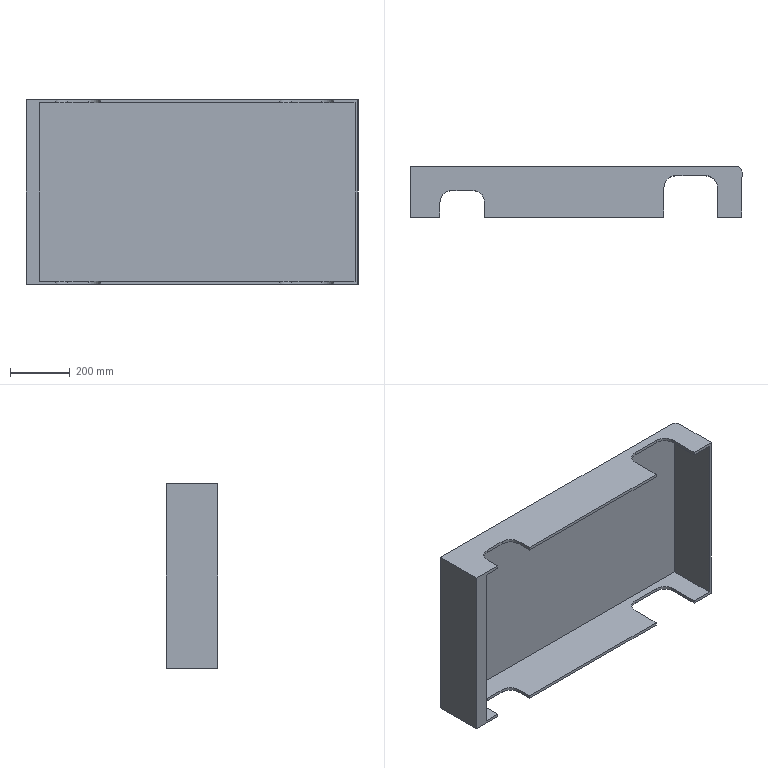Part | SolidWorks | features BaseBody 1 | 1 solid | 35 faces | box 1112 x 170.835 x 618 mm | volume 11764605 mm3 | plane 26 | cylinder 7 | spline 2 | commonest cylinder face diameters 80 x6 40 x1
STEP:
#1=CARTESIAN_POINT('',(484.869,182.944,299.));
#2=VERTEX_POINT('',#1);
#3=CARTESIAN_POINT('',(-571.782,182.944,299.));
#4=VERTEX_POINT('',#3);
#5=CARTESIAN_POINT('',(494.869,182.944,299.));
#6=DIRECTION('',(-1.,0.,0.));
#7=VECTOR('',#6,1000.);
#8=LINE('',#5,#7);
#9=EDGE_CURVE('',#2,#4,#8,.T.);
#10=ORIENTED_EDGE('',*,*,#9,.T.);
#11=CARTESIAN_POINT('',(-571.782,182.944,-299.));
#12=VERTEX_POINT('',#11);
#13=CARTESIAN_POINT('',(-571.782,182.944,-360.));
#14=DIRECTION('',(0.,0.,-1.));
#15=VECTOR('',#14,1000.);
#16=LINE('',#13,#15);
#17=EDGE_CURVE('',#4,#12,#16,.T.);
#18=ORIENTED_EDGE('',*,*,#17,.T.);
#19=CARTESIAN_POINT('',(484.869,182.944,-299.));
#20=VERTEX_POINT('',#19);
#21=CARTESIAN_POINT('',(494.869,182.944,-299.));
#22=DIRECTION('',(-1.,0.,0.));
#23=VECTOR('',#22,1000.);
#24=LINE('',#21,#23);
#25=EDGE_CURVE('',#20,#12,#24,.T.);
#26=ORIENTED_EDGE('',*,*,#25,.F.);
#27=CARTESIAN_POINT('',(484.869,182.944,-360.));
#28=DIRECTION('',(0.,0.,1.));
#29=VECTOR('',#28,1000.);
#30=LINE('',#27,#29);
#31=EDGE_CURVE('',#20,#2,#30,.T.);
#32=ORIENTED_EDGE('',*,*,#31,.T.);
#33=EDGE_LOOP('',(#10,#18,#26,#32));
#34=FACE_OUTER_BOUND('',#33,.T.);
#35=CARTESIAN_POINT('',(494.869,182.944,-360.));
#36=DIRECTION('',(0.,1.,0.));
#37=DIRECTION('',(0.,0.,1.));
#38=AXIS2_PLACEMENT_3D('',#35,#36,#37);
#39=PLANE('',#38);
#40=ADVANCED_FACE('',(#34),#39,.F.);
#41=ORIENTED_EDGE('',*,*,#17,.F.);
#42=CARTESIAN_POINT('',(-571.782,17.142,299.));
#43=VERTEX_POINT('',#42);
#44=CARTESIAN_POINT('',(-571.782,717.138,299.));
#45=DIRECTION('',(0.,-1.,0.));
#46=VECTOR('',#45,1000.);
#47=LINE('',#44,#46);
#48=EDGE_CURVE('',#4,#43,#47,.T.);
#49=ORIENTED_EDGE('',*,*,#48,.T.);
#50=CARTESIAN_POINT('',(-571.782,17.142,-299.));
#51=VERTEX_POINT('',#50);
#52=CARTESIAN_POINT('',(-571.782,17.142,-360.));
#53=DIRECTION('',(0.,0.,1.));
#54=VECTOR('',#53,1000.);
#55=LINE('',#52,#54);
#56=EDGE_CURVE('',#51,#43,#55,.T.);
#57=ORIENTED_EDGE('',*,*,#56,.F.);
#58=CARTESIAN_POINT('',(-571.782,717.138,-299.));
#59=DIRECTION('',(0.,-1.,0.));
#60=VECTOR('',#59,1000.);
#61=LINE('',#58,#60);
#62=EDGE_CURVE('',#12,#51,#61,.T.);
#63=ORIENTED_EDGE('',*,*,#62,.F.);
#64=EDGE_LOOP('',(#41,#49,#57,#63));
#65=FACE_OUTER_BOUND('',#64,.T.);
#66=CARTESIAN_POINT('',(-571.782,717.138,-360.));
#67=DIRECTION('',(-1.,0.,0.));
#68=DIRECTION('',(0.,-1.,0.));
#69=AXIS2_PLACEMENT_3D('',#66,#67,#68);
#70=PLANE('',#69);
#71=ADVANCED_FACE('',(#65),#70,.F.);
#72=CARTESIAN_POINT('',(-616.782,187.944,309.));
#73=VERTEX_POINT('',#72);
#74=CARTESIAN_POINT('',(-616.782,17.108,309.));
#75=VERTEX_POINT('',#74);
#76=CARTESIAN_POINT('',(-616.782,717.138,309.));
#77=DIRECTION('',(0.,-1.,0.));
#78=VECTOR('',#77,1000.);
#79=LINE('',#76,#78);
#80=EDGE_CURVE('',#73,#75,#79,.T.);
#81=ORIENTED_EDGE('',*,*,#80,.F.);
#82=CARTESIAN_POINT('',(-616.782,187.944,-309.));
#83=VERTEX_POINT('',#82);
#84=CARTESIAN_POINT('',(-616.782,187.944,-360.));
#85=DIRECTION('',(0.,0.,-1.));
#86=VECTOR('',#85,1000.);
#87=LINE('',#84,#86);
#88=EDGE_CURVE('',#73,#83,#87,.T.);
#89=ORIENTED_EDGE('',*,*,#88,.T.);
#90=CARTESIAN_POINT('',(-616.782,17.108,-309.));
#91=VERTEX_POINT('',#90);
#92=CARTESIAN_POINT('',(-616.782,717.138,-309.));
#93=DIRECTION('',(0.,-1.,0.));
#94=VECTOR('',#93,1000.);
#95=LINE('',#92,#94);
#96=EDGE_CURVE('',#83,#91,#95,.T.);
#97=ORIENTED_EDGE('',*,*,#96,.T.);
#98=CARTESIAN_POINT('',(-616.782,17.108,-360.));
#99=DIRECTION('',(0.,0.,1.));
#100=VECTOR('',#99,1000.);
#101=LINE('',#98,#100);
#102=EDGE_CURVE('',#91,#75,#101,.T.);
#103=ORIENTED_EDGE('',*,*,#102,.T.);
#104=EDGE_LOOP('',(#81,#89,#97,#103));
#105=FACE_OUTER_BOUND('',#104,.T.);
#106=CARTESIAN_POINT('',(-616.782,717.138,-360.));
#107=DIRECTION('',(-1.,0.,0.));
#108=DIRECTION('',(0.,-1.,0.));
#109=AXIS2_PLACEMENT_3D('',#106,#107,#108);
#110=PLANE('',#109);
#111=ADVANCED_FACE('',(#105),#110,.T.);
#112=CARTESIAN_POINT('',(474.869,187.944,309.));
#113=VERTEX_POINT('',#112);
#114=CARTESIAN_POINT('',(494.869,187.944,309.));
#115=DIRECTION('',(-1.,0.,0.));
#116=VECTOR('',#115,1000.);
#117=LINE('',#114,#116);
#118=EDGE_CURVE('',#113,#73,#117,.T.);
#119=ORIENTED_EDGE('',*,*,#118,.T.);
#120=ORIENTED_EDGE('',*,*,#80,.T.);
#121=CARTESIAN_POINT('',(-516.782,17.183,309.));
#122=VERTEX_POINT('',#121);
#123=CARTESIAN_POINT('',(-576.782,17.138,309.));
#124=DIRECTION('',(1.,0.0007515,0.));
#125=VECTOR('',#124,1000.);
#126=LINE('',#123,#125);
#127=EDGE_CURVE('',#75,#122,#126,.T.);
#128=ORIENTED_EDGE('',*,*,#127,.T.);
#129=CARTESIAN_POINT('',(-516.782,67.138,309.));
#130=VERTEX_POINT('',#129);
#131=CARTESIAN_POINT('',(-516.782,0.,309.));
#132=DIRECTION('',(0.,-1.,0.));
#133=VECTOR('',#132,1000.);
#134=LINE('',#131,#133);
#135=EDGE_CURVE('',#130,#122,#134,.T.);
#136=ORIENTED_EDGE('',*,*,#135,.F.);
#137=CARTESIAN_POINT('',(-476.782,107.138,309.));
#138=VERTEX_POINT('',#137);
#139=CARTESIAN_POINT('',(-476.782,67.138,309.));
#140=DIRECTION('',(0.,0.,1.));
#141=DIRECTION('',(-1.,0.,0.));
#142=AXIS2_PLACEMENT_3D('',#139,#140,#141);
#143=CIRCLE('',#142,40.);
#144=EDGE_CURVE('',#138,#130,#143,.T.);
#145=ORIENTED_EDGE('',*,*,#144,.F.);
#146=CARTESIAN_POINT('',(-406.782,107.138,309.));
#147=VERTEX_POINT('',#146);
#148=CARTESIAN_POINT('',(0.,107.138,309.));
#149=DIRECTION('',(-1.,0.,0.));
#150=VECTOR('',#149,1000.);
#151=LINE('',#148,#150);
#152=EDGE_CURVE('',#147,#138,#151,.T.);
#153=ORIENTED_EDGE('',*,*,#152,.F.);
#154=CARTESIAN_POINT('',(-366.782,67.138,309.));
#155=VERTEX_POINT('',#154);
#156=CARTESIAN_POINT('',(-406.782,67.138,309.));
#157=DIRECTION('',(0.,0.,1.));
#158=DIRECTION('',(-1.,0.,0.));
#159=AXIS2_PLACEMENT_3D('',#156,#157,#158);
#160=CIRCLE('',#159,40.);
#161=EDGE_CURVE('',#155,#147,#160,.T.);
#162=ORIENTED_EDGE('',*,*,#161,.F.);
#163=CARTESIAN_POINT('',(-366.782,17.296,309.));
#164=VERTEX_POINT('',#163);
#165=CARTESIAN_POINT('',(-366.782,0.,309.));
#166=DIRECTION('',(0.,1.,0.));
#167=VECTOR('',#166,1000.);
#168=LINE('',#165,#167);
#169=EDGE_CURVE('',#164,#155,#168,.T.);
#170=ORIENTED_EDGE('',*,*,#169,.F.);
#171=CARTESIAN_POINT('',(233.218,17.747,309.));
#172=VERTEX_POINT('',#171);
#173=CARTESIAN_POINT('',(-576.782,17.138,309.));
#174=DIRECTION('',(1.,0.0007515,0.));
#175=VECTOR('',#174,1000.);
#176=LINE('',#173,#175);
#177=EDGE_CURVE('',#164,#172,#176,.T.);
#178=ORIENTED_EDGE('',*,*,#177,.T.);
#179=CARTESIAN_POINT('',(233.218,117.138,309.));
#180=VERTEX_POINT('',#179);
#181=CARTESIAN_POINT('',(233.218,0.,309.));
#182=DIRECTION('',(0.,-1.,0.));
#183=VECTOR('',#182,1000.);
#184=LINE('',#181,#183);
#185=EDGE_CURVE('',#180,#172,#184,.T.);
#186=ORIENTED_EDGE('',*,*,#185,.F.);
#187=CARTESIAN_POINT('',(273.218,157.138,309.));
#188=VERTEX_POINT('',#187);
#189=CARTESIAN_POINT('',(273.218,117.138,309.));
#190=DIRECTION('',(0.,0.,1.));
#191=DIRECTION('',(-1.,0.,0.));
#192=AXIS2_PLACEMENT_3D('',#189,#190,#191);
#193=CIRCLE('',#192,40.);
#194=EDGE_CURVE('',#188,#180,#193,.T.);
#195=ORIENTED_EDGE('',*,*,#194,.F.);
#196=CARTESIAN_POINT('',(373.218,157.138,309.));
#197=VERTEX_POINT('',#196);
#198=CARTESIAN_POINT('',(0.,157.138,309.));
#199=DIRECTION('',(-1.,0.,0.));
#200=VECTOR('',#199,1000.);
#201=LINE('',#198,#200);
#202=EDGE_CURVE('',#197,#188,#201,.T.);
#203=ORIENTED_EDGE('',*,*,#202,.F.);
#204=CARTESIAN_POINT('',(413.218,117.138,309.));
#205=VERTEX_POINT('',#204);
#206=CARTESIAN_POINT('',(413.218,117.138,309.));
#207=CARTESIAN_POINT('',(413.218,119.8,309.));
#208=CARTESIAN_POINT('',(412.955,122.414,309.));
#209=CARTESIAN_POINT('',(412.185,126.265,309.));
#210=CARTESIAN_POINT('',(411.865,127.537,309.));
#211=CARTESIAN_POINT('',(411.289,129.428,309.));
#212=CARTESIAN_POINT('',(411.08,130.057,309.));
#213=CARTESIAN_POINT('',(410.634,131.297,309.));
#214=CARTESIAN_POINT('',(410.396,131.909,309.));
#215=CARTESIAN_POINT('',(409.139,134.929,309.));
#216=CARTESIAN_POINT('',(407.911,137.217,309.));
#217=CARTESIAN_POINT('',(406.1,139.924,309.));
#218=CARTESIAN_POINT('',(405.724,140.458,309.));
#219=CARTESIAN_POINT('',(404.943,141.51,309.));
#220=CARTESIAN_POINT('',(404.539,142.026,309.));
#221=CARTESIAN_POINT('',(403.297,143.538,309.));
#222=CARTESIAN_POINT('',(402.426,144.498,309.));
#223=CARTESIAN_POINT('',(400.597,146.328,309.));
#224=CARTESIAN_POINT('',(399.639,147.198,309.));
#225=CARTESIAN_POINT('',(397.637,148.846,309.));
#226=CARTESIAN_POINT('',(396.592,149.625,309.));
#227=CARTESIAN_POINT('',(394.41,151.088,309.));
#228=CARTESIAN_POINT('',(393.29,151.762,309.));
#229=CARTESIAN_POINT('',(390.998,152.993,309.));
#230=CARTESIAN_POINT('',(389.824,153.551,309.));
#231=CARTESIAN_POINT('',(387.423,154.554,309.));
#232=CARTESIAN_POINT('',(386.195,154.998,309.));
#233=CARTESIAN_POINT('',(384.311,155.575,309.));
#234=CARTESIAN_POINT('',(383.675,155.753,309.));
#235=CARTESIAN_POINT('',(382.39,156.078,309.));
#236=CARTESIAN_POINT('',(381.744,156.225,309.));
#237=CARTESIAN_POINT('',(378.505,156.875,309.));
#238=CARTESIAN_POINT('',(375.879,157.138,309.));
#239=CARTESIAN_POINT('',(373.218,157.138,309.));
#240=B_SPLINE_CURVE_WITH_KNOTS('',3,(#206,#207,#208,#209,#210,#211,#212,#213,#214,#215,#216,#217,#218,#219,#220,#221,#222,#223,#224,#225,#226,#227,#228,#229,#230,#231,#232,#233,#234,#235,#236,#237,#238,#239),.UNSPECIFIED.,.F.,.F.,(4,2,2,2,2,2,2,2,2,2,2,2,2,2,2,2,4),(0.,0.125,0.1875,0.2187,0.25,0.375,0.4062,0.4375,0.5,0.5625,0.625,0.6875,0.75,0.8125,0.8438,0.875,1.),.UNSPECIFIED.);
#241=EDGE_CURVE('',#205,#197,#240,.T.);
#242=ORIENTED_EDGE('',*,*,#241,.F.);
#243=CARTESIAN_POINT('',(413.218,17.882,309.));
#244=VERTEX_POINT('',#243);
#245=CARTESIAN_POINT('',(413.218,0.,309.));
#246=DIRECTION('',(0.,1.,0.));
#247=VECTOR('',#246,1000.);
#248=LINE('',#245,#247);
#249=EDGE_CURVE('',#244,#205,#248,.T.);
#250=ORIENTED_EDGE('',*,*,#249,.F.);
#251=CARTESIAN_POINT('',(494.869,17.944,309.));
#252=VERTEX_POINT('',#251);
#253=CARTESIAN_POINT('',(-576.782,17.138,309.));
#254=DIRECTION('',(1.,0.0007515,0.));
#255=VECTOR('',#254,1000.);
#256=LINE('',#253,#255);
#257=EDGE_CURVE('',#244,#252,#256,.T.);
#258=ORIENTED_EDGE('',*,*,#257,.T.);
#259=CARTESIAN_POINT('',(494.869,167.944,309.));
#260=VERTEX_POINT('',#259);
#261=CARTESIAN_POINT('',(494.869,17.944,309.));
#262=DIRECTION('',(0.,1.,0.));
#263=VECTOR('',#262,1000.);
#264=LINE('',#261,#263);
#265=EDGE_CURVE('',#252,#260,#264,.T.);
#266=ORIENTED_EDGE('',*,*,#265,.T.);
#267=CARTESIAN_POINT('',(474.869,167.944,309.));
#268=DIRECTION('',(0.,0.,1.));
#269=DIRECTION('',(-1.,0.,0.));
#270=AXIS2_PLACEMENT_3D('',#267,#268,#269);
#271=CIRCLE('',#270,20.);
#272=EDGE_CURVE('',#260,#113,#271,.T.);
#273=ORIENTED_EDGE('',*,*,#272,.T.);
#274=EDGE_LOOP('',(#119,#120,#128,#136,#145,#153,#162,#170,#178,#186,#195,#203,#242,#250,#258,#266,#273));
#275=FACE_OUTER_BOUND('',#274,.T.);
#276=CARTESIAN_POINT('',(0.,0.,309.));
#277=DIRECTION('',(0.,0.,-1.));
#278=DIRECTION('',(-1.,0.,0.));
#279=AXIS2_PLACEMENT_3D('',#276,#277,#278);
#280=PLANE('',#279);
#281=ADVANCED_FACE('',(#275),#280,.F.);
#282=ORIENTED_EDGE('',*,*,#96,.F.);
#283=CARTESIAN_POINT('',(474.869,187.944,-309.));
#284=VERTEX_POINT('',#283);
#285=CARTESIAN_POINT('',(494.869,187.944,-309.));
#286=DIRECTION('',(-1.,0.,0.));
#287=VECTOR('',#286,1000.);
#288=LINE('',#285,#287);
#289=EDGE_CURVE('',#284,#83,#288,.T.);
#290=ORIENTED_EDGE('',*,*,#289,.F.);
#291=CARTESIAN_POINT('',(494.869,167.944,-309.));
#292=VERTEX_POINT('',#291);
#293=CARTESIAN_POINT('',(474.869,167.944,-309.));
#294=DIRECTION('',(0.,0.,-1.));
#295=DIRECTION('',(-1.,0.,0.));
#296=AXIS2_PLACEMENT_3D('',#293,#294,#295);
#297=CIRCLE('',#296,20.);
#298=EDGE_CURVE('',#284,#292,#297,.T.);
#299=ORIENTED_EDGE('',*,*,#298,.T.);
#300=CARTESIAN_POINT('',(494.869,17.944,-309.));
#301=VERTEX_POINT('',#300);
#302=CARTESIAN_POINT('',(494.869,17.944,-309.));
#303=DIRECTION('',(0.,1.,0.));
#304=VECTOR('',#303,1000.);
#305=LINE('',#302,#304);
#306=EDGE_CURVE('',#301,#292,#305,.T.);
#307=ORIENTED_EDGE('',*,*,#306,.F.);
#308=CARTESIAN_POINT('',(413.218,17.882,-309.));
#309=VERTEX_POINT('',#308);
#310=CARTESIAN_POINT('',(-576.782,17.138,-309.));
#311=DIRECTION('',(1.,0.0007515,0.));
#312=VECTOR('',#311,1000.);
#313=LINE('',#310,#312);
#314=EDGE_CURVE('',#309,#301,#313,.T.);
#315=ORIENTED_EDGE('',*,*,#314,.F.);
#316=CARTESIAN_POINT('',(413.218,117.138,-309.));
#317=VERTEX_POINT('',#316);
#318=CARTESIAN_POINT('',(413.218,7.138,-309.));
#319=DIRECTION('',(0.,1.,0.));
#320=VECTOR('',#319,1000.);
#321=LINE('',#318,#320);
#322=EDGE_CURVE('',#309,#317,#321,.T.);
#323=ORIENTED_EDGE('',*,*,#322,.T.);
#324=CARTESIAN_POINT('',(373.218,157.138,-309.));
#325=VERTEX_POINT('',#324);
#326=CARTESIAN_POINT('',(413.218,117.138,-309.));
#327=CARTESIAN_POINT('',(413.218,119.8,-309.));
#328=CARTESIAN_POINT('',(412.955,122.414,-309.));
#329=CARTESIAN_POINT('',(412.185,126.265,-309.));
#330=CARTESIAN_POINT('',(411.865,127.537,-309.));
#331=CARTESIAN_POINT('',(411.289,129.428,-309.));
#332=CARTESIAN_POINT('',(411.08,130.057,-309.));
#333=CARTESIAN_POINT('',(410.634,131.297,-309.));
#334=CARTESIAN_POINT('',(410.396,131.909,-309.));
#335=CARTESIAN_POINT('',(409.139,134.929,-309.));
#336=CARTESIAN_POINT('',(407.911,137.217,-309.));
#337=CARTESIAN_POINT('',(406.1,139.924,-309.));
#338=CARTESIAN_POINT('',(405.724,140.458,-309.));
#339=CARTESIAN_POINT('',(404.943,141.51,-309.));
#340=CARTESIAN_POINT('',(404.539,142.026,-309.));
#341=CARTESIAN_POINT('',(403.297,143.538,-309.));
#342=CARTESIAN_POINT('',(402.426,144.498,-309.));
#343=CARTESIAN_POINT('',(400.597,146.328,-309.));
#344=CARTESIAN_POINT('',(399.639,147.198,-309.));
#345=CARTESIAN_POINT('',(397.637,148.846,-309.));
#346=CARTESIAN_POINT('',(396.592,149.625,-309.));
#347=CARTESIAN_POINT('',(394.41,151.088,-309.));
#348=CARTESIAN_POINT('',(393.29,151.762,-309.));
#349=CARTESIAN_POINT('',(390.998,152.993,-309.));
#350=CARTESIAN_POINT('',(389.824,153.551,-309.));
#351=CARTESIAN_POINT('',(387.423,154.554,-309.));
#352=CARTESIAN_POINT('',(386.195,154.998,-309.));
#353=CARTESIAN_POINT('',(384.311,155.575,-309.));
#354=CARTESIAN_POINT('',(383.675,155.753,-309.));
#355=CARTESIAN_POINT('',(382.39,156.078,-309.));
#356=CARTESIAN_POINT('',(381.744,156.225,-309.));
#357=CARTESIAN_POINT('',(378.505,156.875,-309.));
#358=CARTESIAN_POINT('',(375.879,157.138,-309.));
#359=CARTESIAN_POINT('',(373.218,157.138,-309.));
#360=B_SPLINE_CURVE_WITH_KNOTS('',3,(#326,#327,#328,#329,#330,#331,#332,#333,#334,#335,#336,#337,#338,#339,#340,#341,#342,#343,#344,#345,#346,#347,#348,#349,#350,#351,#352,#353,#354,#355,#356,#357,#358,#359),.UNSPECIFIED.,.F.,.F.,(4,2,2,2,2,2,2,2,2,2,2,2,2,2,2,2,4),(0.,0.125,0.1875,0.2187,0.25,0.375,0.4062,0.4375,0.5,0.5625,0.625,0.6875,0.75,0.8125,0.8438,0.875,1.),.UNSPECIFIED.);
#361=EDGE_CURVE('',#317,#325,#360,.T.);
#362=ORIENTED_EDGE('',*,*,#361,.T.);
#363=CARTESIAN_POINT('',(273.218,157.138,-309.));
#364=VERTEX_POINT('',#363);
#365=CARTESIAN_POINT('',(373.218,157.138,-309.));
#366=DIRECTION('',(-1.,0.,0.));
#367=VECTOR('',#366,1000.);
#368=LINE('',#365,#367);
#369=EDGE_CURVE('',#325,#364,#368,.T.);
#370=ORIENTED_EDGE('',*,*,#369,.T.);
#371=CARTESIAN_POINT('',(233.218,117.138,-309.));
#372=VERTEX_POINT('',#371);
#373=CARTESIAN_POINT('',(273.218,117.138,-309.));
#374=DIRECTION('',(0.,0.,1.));
#375=DIRECTION('',(1.,0.,0.));
#376=AXIS2_PLACEMENT_3D('',#373,#374,#375);
#377=CIRCLE('',#376,40.);
#378=EDGE_CURVE('',#364,#372,#377,.T.);
#379=ORIENTED_EDGE('',*,*,#378,.T.);
#380=CARTESIAN_POINT('',(233.218,17.747,-309.));
#381=VERTEX_POINT('',#380);
#382=CARTESIAN_POINT('',(233.218,17.138,-309.));
#383=DIRECTION('',(0.,-1.,0.));
#384=VECTOR('',#383,1000.);
#385=LINE('',#382,#384);
#386=EDGE_CURVE('',#372,#381,#385,.T.);
#387=ORIENTED_EDGE('',*,*,#386,.T.);
#388=CARTESIAN_POINT('',(-366.782,17.296,-309.));
#389=VERTEX_POINT('',#388);
#390=CARTESIAN_POINT('',(-576.782,17.138,-309.));
#391=DIRECTION('',(1.,0.0007515,0.));
#392=VECTOR('',#391,1000.);
#393=LINE('',#390,#392);
#394=EDGE_CURVE('',#389,#381,#393,.T.);
#395=ORIENTED_EDGE('',*,*,#394,.F.);
#396=CARTESIAN_POINT('',(-366.782,67.138,-309.));
#397=VERTEX_POINT('',#396);
#398=CARTESIAN_POINT('',(-366.782,17.138,-309.));
#399=DIRECTION('',(0.,1.,0.));
#400=VECTOR('',#399,1000.);
#401=LINE('',#398,#400);
#402=EDGE_CURVE('',#389,#397,#401,.T.);
#403=ORIENTED_EDGE('',*,*,#402,.T.);
#404=CARTESIAN_POINT('',(-406.782,107.138,-309.));
#405=VERTEX_POINT('',#404);
#406=CARTESIAN_POINT('',(-406.782,67.138,-309.));
#407=DIRECTION('',(0.,0.,1.));
#408=DIRECTION('',(1.,0.,0.));
#409=AXIS2_PLACEMENT_3D('',#406,#407,#408);
#410=CIRCLE('',#409,40.);
#411=EDGE_CURVE('',#397,#405,#410,.T.);
#412=ORIENTED_EDGE('',*,*,#411,.T.);
#413=CARTESIAN_POINT('',(-476.782,107.138,-309.));
#414=VERTEX_POINT('',#413);
#415=CARTESIAN_POINT('',(-406.782,107.138,-309.));
#416=DIRECTION('',(-1.,0.,0.));
#417=VECTOR('',#416,1000.);
#418=LINE('',#415,#417);
#419=EDGE_CURVE('',#405,#414,#418,.T.);
#420=ORIENTED_EDGE('',*,*,#419,.T.);
#421=CARTESIAN_POINT('',(-516.782,67.138,-309.));
#422=VERTEX_POINT('',#421);
#423=CARTESIAN_POINT('',(-476.782,67.138,-309.));
#424=DIRECTION('',(0.,0.,1.));
#425=DIRECTION('',(1.,0.,0.));
#426=AXIS2_PLACEMENT_3D('',#423,#424,#425);
#427=CIRCLE('',#426,40.);
#428=EDGE_CURVE('',#414,#422,#427,.T.);
#429=ORIENTED_EDGE('',*,*,#428,.T.);
#430=CARTESIAN_POINT('',(-516.782,17.183,-309.));
#431=VERTEX_POINT('',#430);
#432=CARTESIAN_POINT('',(-516.782,17.138,-309.));
#433=DIRECTION('',(0.,-1.,0.));
#434=VECTOR('',#433,1000.);
#435=LINE('',#432,#434);
#436=EDGE_CURVE('',#422,#431,#435,.T.);
#437=ORIENTED_EDGE('',*,*,#436,.T.);
#438=CARTESIAN_POINT('',(-576.782,17.138,-309.));
#439=DIRECTION('',(1.,0.0007515,0.));
#440=VECTOR('',#439,1000.);
#441=LINE('',#438,#440);
#442=EDGE_CURVE('',#91,#431,#441,.T.);
#443=ORIENTED_EDGE('',*,*,#442,.F.);
#444=EDGE_LOOP('',(#282,#290,#299,#307,#315,#323,#362,#370,#379,#387,#395,#403,#412,#420,#429,#437,#443));
#445=FACE_OUTER_BOUND('',#444,.T.);
#446=CARTESIAN_POINT('',(0.,0.,-309.));
#447=DIRECTION('',(0.,0.,-1.));
#448=DIRECTION('',(-1.,0.,0.));
#449=AXIS2_PLACEMENT_3D('',#446,#447,#448);
#450=PLANE('',#449);
#451=ADVANCED_FACE('',(#445),#450,.T.);
#452=ORIENTED_EDGE('',*,*,#25,.T.);
#453=ORIENTED_EDGE('',*,*,#62,.T.);
#454=CARTESIAN_POINT('',(-516.782,17.183,-299.));
#455=VERTEX_POINT('',#454);
#456=CARTESIAN_POINT('',(-576.782,17.138,-299.));
#457=DIRECTION('',(1.,0.0007515,0.));
#458=VECTOR('',#457,1000.);
#459=LINE('',#456,#458);
#460=EDGE_CURVE('',#51,#455,#459,.T.);
#461=ORIENTED_EDGE('',*,*,#460,.T.);
#462=CARTESIAN_POINT('',(-516.782,67.138,-299.));
#463=VERTEX_POINT('',#462);
#464=CARTESIAN_POINT('',(-516.782,0.,-299.));
#465=DIRECTION('',(0.,-1.,0.));
#466=VECTOR('',#465,1000.);
#467=LINE('',#464,#466);
#468=EDGE_CURVE('',#463,#455,#467,.T.);
#469=ORIENTED_EDGE('',*,*,#468,.F.);
#470=CARTESIAN_POINT('',(-476.782,107.138,-299.));
#471=VERTEX_POINT('',#470);
#472=CARTESIAN_POINT('',(-476.782,67.138,-299.));
#473=DIRECTION('',(0.,0.,1.));
#474=DIRECTION('',(-1.,0.,0.));
#475=AXIS2_PLACEMENT_3D('',#472,#473,#474);
#476=CIRCLE('',#475,40.);
#477=EDGE_CURVE('',#471,#463,#476,.T.);
#478=ORIENTED_EDGE('',*,*,#477,.F.);
#479=CARTESIAN_POINT('',(-406.782,107.138,-299.));
#480=VERTEX_POINT('',#479);
#481=CARTESIAN_POINT('',(0.,107.138,-299.));
#482=DIRECTION('',(-1.,0.,0.));
#483=VECTOR('',#482,1000.);
#484=LINE('',#481,#483);
#485=EDGE_CURVE('',#480,#471,#484,.T.);
#486=ORIENTED_EDGE('',*,*,#485,.F.);
#487=CARTESIAN_POINT('',(-366.782,67.138,-299.));
#488=VERTEX_POINT('',#487);
#489=CARTESIAN_POINT('',(-406.782,67.138,-299.));
#490=DIRECTION('',(0.,0.,1.));
#491=DIRECTION('',(-1.,0.,0.));
#492=AXIS2_PLACEMENT_3D('',#489,#490,#491);
#493=CIRCLE('',#492,40.);
#494=EDGE_CURVE('',#488,#480,#493,.T.);
#495=ORIENTED_EDGE('',*,*,#494,.F.);
#496=CARTESIAN_POINT('',(-366.782,17.296,-299.));
#497=VERTEX_POINT('',#496);
#498=CARTESIAN_POINT('',(-366.782,0.,-299.));
#499=DIRECTION('',(0.,1.,0.));
#500=VECTOR('',#499,1000.);
#501=LINE('',#498,#500);
#502=EDGE_CURVE('',#497,#488,#501,.T.);
#503=ORIENTED_EDGE('',*,*,#502,.F.);
#504=CARTESIAN_POINT('',(233.218,17.747,-299.));
#505=VERTEX_POINT('',#504);
#506=CARTESIAN_POINT('',(-576.782,17.138,-299.));
#507=DIRECTION('',(1.,0.0007515,0.));
#508=VECTOR('',#507,1000.);
#509=LINE('',#506,#508);
#510=EDGE_CURVE('',#497,#505,#509,.T.);
#511=ORIENTED_EDGE('',*,*,#510,.T.);
#512=CARTESIAN_POINT('',(233.218,117.138,-299.));
#513=VERTEX_POINT('',#512);
#514=CARTESIAN_POINT('',(233.218,0.,-299.));
#515=DIRECTION('',(0.,-1.,0.));
#516=VECTOR('',#515,1000.);
#517=LINE('',#514,#516);
#518=EDGE_CURVE('',#513,#505,#517,.T.);
#519=ORIENTED_EDGE('',*,*,#518,.F.);
#520=CARTESIAN_POINT('',(273.218,157.138,-299.));
#521=VERTEX_POINT('',#520);
#522=CARTESIAN_POINT('',(273.218,117.138,-299.));
#523=DIRECTION('',(0.,0.,1.));
#524=DIRECTION('',(-1.,0.,0.));
#525=AXIS2_PLACEMENT_3D('',#522,#523,#524);
#526=CIRCLE('',#525,40.);
#527=EDGE_CURVE('',#521,#513,#526,.T.);
#528=ORIENTED_EDGE('',*,*,#527,.F.);
#529=CARTESIAN_POINT('',(373.218,157.138,-299.));
#530=VERTEX_POINT('',#529);
#531=CARTESIAN_POINT('',(0.,157.138,-299.));
#532=DIRECTION('',(-1.,0.,0.));
#533=VECTOR('',#532,1000.);
#534=LINE('',#531,#533);
#535=EDGE_CURVE('',#530,#521,#534,.T.);
#536=ORIENTED_EDGE('',*,*,#535,.F.);
#537=CARTESIAN_POINT('',(413.218,117.138,-299.));
#538=VERTEX_POINT('',#537);
#539=CARTESIAN_POINT('',(413.218,117.138,-299.));
#540=CARTESIAN_POINT('',(413.218,119.761,-299.));
#541=CARTESIAN_POINT('',(412.962,122.351,-299.));
#542=CARTESIAN_POINT('',(412.202,126.191,-299.));
#543=CARTESIAN_POINT('',(411.885,127.463,-299.));
#544=CARTESIAN_POINT('',(411.311,129.358,-299.));
#545=CARTESIAN_POINT('',(411.104,129.985,-299.));
#546=CARTESIAN_POINT('',(410.662,131.222,-299.));
#547=CARTESIAN_POINT('',(410.427,131.832,-299.));
#548=CARTESIAN_POINT('',(409.179,134.848,-299.));
#549=CARTESIAN_POINT('',(407.956,137.14,-299.));
#550=CARTESIAN_POINT('',(406.146,139.857,-299.));
#551=CARTESIAN_POINT('',(405.77,140.393,-299.));
#552=CARTESIAN_POINT('',(404.989,141.45,-299.));
#553=CARTESIAN_POINT('',(404.583,141.971,-299.));
#554=CARTESIAN_POINT('',(403.327,143.505,-299.));
#555=CARTESIAN_POINT('',(402.438,144.486,-299.));
#556=CARTESIAN_POINT('',(399.659,147.267,-299.));
#557=CARTESIAN_POINT('',(397.644,148.922,-299.));
#558=CARTESIAN_POINT('',(394.925,150.742,-299.));
#559=CARTESIAN_POINT('',(394.371,151.094,-299.));
#560=CARTESIAN_POINT('',(393.243,151.771,-299.));
#561=CARTESIAN_POINT('',(392.667,152.098,-299.));
#562=CARTESIAN_POINT('',(390.924,153.03,-299.));
#563=CARTESIAN_POINT('',(389.739,153.59,-299.));
#564=CARTESIAN_POINT('',(386.123,155.089,-299.));
#565=CARTESIAN_POINT('',(383.626,155.85,-299.));
#566=CARTESIAN_POINT('',(380.397,156.494,-299.));
#567=CARTESIAN_POINT('',(379.744,156.608,-299.));
#568=CARTESIAN_POINT('',(378.441,156.802,-299.));
#569=CARTESIAN_POINT('',(376.485,157.043,-299.));
#570=CARTESIAN_POINT('',(374.526,157.138,-299.));
#571=CARTESIAN_POINT('',(373.218,157.138,-299.));
#572=B_SPLINE_CURVE_WITH_KNOTS('',3,(#539,#540,#541,#542,#543,#544,#545,#546,#547,#548,#549,#550,#551,#552,#553,#554,#555,#556,#557,#558,#559,#560,#561,#562,#563,#564,#565,#566,#567,#568,#569,#570,#571),.UNSPECIFIED.,.F.,.F.,(4,2,2,2,2,2,2,2,2,2,2,2,2,2,2,1,4),(0.1304,0.1383,0.1422,0.1442,0.1462,0.154,0.156,0.158,0.1619,0.1698,0.1718,0.1737,0.1777,0.1855,0.1875,0.1895,0.1934),.UNSPECIFIED.);
#573=EDGE_CURVE('',#538,#530,#572,.T.);
#574=ORIENTED_EDGE('',*,*,#573,.F.);
#575=CARTESIAN_POINT('',(413.218,17.882,-299.));
#576=VERTEX_POINT('',#575);
#577=CARTESIAN_POINT('',(413.218,0.,-299.));
#578=DIRECTION('',(0.,1.,0.));
#579=VECTOR('',#578,1000.);
#580=LINE('',#577,#579);
#581=EDGE_CURVE('',#576,#538,#580,.T.);
#582=ORIENTED_EDGE('',*,*,#581,.F.);
#583=CARTESIAN_POINT('',(484.869,17.936,-299.));
#584=VERTEX_POINT('',#583);
#585=CARTESIAN_POINT('',(-576.782,17.138,-299.));
#586=DIRECTION('',(1.,0.0007515,0.));
#587=VECTOR('',#586,1000.);
#588=LINE('',#585,#587);
#589=EDGE_CURVE('',#576,#584,#588,.T.);
#590=ORIENTED_EDGE('',*,*,#589,.T.);
#591=CARTESIAN_POINT('',(484.869,17.944,-299.));
#592=DIRECTION('',(0.,1.,0.));
#593=VECTOR('',#592,1000.);
#594=LINE('',#591,#593);
#595=EDGE_CURVE('',#584,#20,#594,.T.);
#596=ORIENTED_EDGE('',*,*,#595,.T.);
#597=EDGE_LOOP('',(#452,#453,#461,#469,#478,#486,#495,#503,#511,#519,#528,#536,#574,#582,#590,#596));
#598=FACE_OUTER_BOUND('',#597,.T.);
#599=CARTESIAN_POINT('',(0.,0.,-299.));
#600=DIRECTION('',(0.,0.,-1.));
#601=DIRECTION('',(-1.,0.,0.));
#602=AXIS2_PLACEMENT_3D('',#599,#600,#601);
#603=PLANE('',#602);
#604=ADVANCED_FACE('',(#598),#603,.F.);
#605=ORIENTED_EDGE('',*,*,#48,.F.);
#606=ORIENTED_EDGE('',*,*,#9,.F.);
#607=CARTESIAN_POINT('',(484.869,17.936,299.));
#608=VERTEX_POINT('',#607);
#609=CARTESIAN_POINT('',(484.869,17.944,299.));
#610=DIRECTION('',(0.,1.,0.));
#611=VECTOR('',#610,1000.);
#612=LINE('',#609,#611);
#613=EDGE_CURVE('',#608,#2,#612,.T.);
#614=ORIENTED_EDGE('',*,*,#613,.F.);
#615=CARTESIAN_POINT('',(413.218,17.882,299.));
#616=VERTEX_POINT('',#615);
#617=CARTESIAN_POINT('',(-576.782,17.138,299.));
#618=DIRECTION('',(1.,0.0007515,0.));
#619=VECTOR('',#618,1000.);
#620=LINE('',#617,#619);
#621=EDGE_CURVE('',#616,#608,#620,.T.);
#622=ORIENTED_EDGE('',*,*,#621,.F.);
#623=CARTESIAN_POINT('',(413.218,117.138,299.));
#624=VERTEX_POINT('',#623);
#625=CARTESIAN_POINT('',(413.218,0.,299.));
#626=DIRECTION('',(0.,1.,0.));
#627=VECTOR('',#626,1000.);
#628=LINE('',#625,#627);
#629=EDGE_CURVE('',#616,#624,#628,.T.);
#630=ORIENTED_EDGE('',*,*,#629,.T.);
#631=CARTESIAN_POINT('',(373.218,157.138,299.));
#632=VERTEX_POINT('',#631);
#633=CARTESIAN_POINT('',(413.218,117.138,299.));
#634=CARTESIAN_POINT('',(413.218,119.761,299.));
#635=CARTESIAN_POINT('',(412.962,122.351,299.));
#636=CARTESIAN_POINT('',(412.202,126.191,299.));
#637=CARTESIAN_POINT('',(411.885,127.463,299.));
#638=CARTESIAN_POINT('',(411.311,129.358,299.));
#639=CARTESIAN_POINT('',(411.104,129.985,299.));
#640=CARTESIAN_POINT('',(410.662,131.222,299.));
#641=CARTESIAN_POINT('',(410.427,131.832,299.));
#642=CARTESIAN_POINT('',(409.179,134.848,299.));
#643=CARTESIAN_POINT('',(407.956,137.14,299.));
#644=CARTESIAN_POINT('',(406.146,139.857,299.));
#645=CARTESIAN_POINT('',(405.77,140.393,299.));
#646=CARTESIAN_POINT('',(404.989,141.45,299.));
#647=CARTESIAN_POINT('',(404.583,141.971,299.));
#648=CARTESIAN_POINT('',(403.327,143.505,299.));
#649=CARTESIAN_POINT('',(402.438,144.486,299.));
#650=CARTESIAN_POINT('',(399.659,147.267,299.));
#651=CARTESIAN_POINT('',(397.644,148.922,299.));
#652=CARTESIAN_POINT('',(394.925,150.742,299.));
#653=CARTESIAN_POINT('',(394.371,151.094,299.));
#654=CARTESIAN_POINT('',(393.243,151.771,299.));
#655=CARTESIAN_POINT('',(392.667,152.098,299.));
#656=CARTESIAN_POINT('',(390.924,153.03,299.));
#657=CARTESIAN_POINT('',(389.739,153.59,299.));
#658=CARTESIAN_POINT('',(386.123,155.089,299.));
#659=CARTESIAN_POINT('',(383.626,155.85,299.));
#660=CARTESIAN_POINT('',(380.397,156.494,299.));
#661=CARTESIAN_POINT('',(379.744,156.608,299.));
#662=CARTESIAN_POINT('',(378.441,156.802,299.));
#663=CARTESIAN_POINT('',(376.485,157.043,299.));
#664=CARTESIAN_POINT('',(374.526,157.138,299.));
#665=CARTESIAN_POINT('',(373.218,157.138,299.));
#666=B_SPLINE_CURVE_WITH_KNOTS('',3,(#633,#634,#635,#636,#637,#638,#639,#640,#641,#642,#643,#644,#645,#646,#647,#648,#649,#650,#651,#652,#653,#654,#655,#656,#657,#658,#659,#660,#661,#662,#663,#664,#665),.UNSPECIFIED.,.F.,.F.,(4,2,2,2,2,2,2,2,2,2,2,2,2,2,2,1,4),(0.1304,0.1383,0.1422,0.1442,0.1462,0.154,0.156,0.158,0.1619,0.1698,0.1718,0.1737,0.1777,0.1855,0.1875,0.1895,0.1934),.UNSPECIFIED.);
#667=EDGE_CURVE('',#624,#632,#666,.T.);
#668=ORIENTED_EDGE('',*,*,#667,.T.);
#669=CARTESIAN_POINT('',(273.218,157.138,299.));
#670=VERTEX_POINT('',#669);
#671=CARTESIAN_POINT('',(0.,157.138,299.));
#672=DIRECTION('',(-1.,0.,0.));
#673=VECTOR('',#672,1000.);
#674=LINE('',#671,#673);
#675=EDGE_CURVE('',#632,#670,#674,.T.);
#676=ORIENTED_EDGE('',*,*,#675,.T.);
#677=CARTESIAN_POINT('',(233.218,117.138,299.));
#678=VERTEX_POINT('',#677);
#679=CARTESIAN_POINT('',(273.218,117.138,299.));
#680=DIRECTION('',(0.,0.,1.));
#681=DIRECTION('',(-1.,0.,0.));
#682=AXIS2_PLACEMENT_3D('',#679,#680,#681);
#683=CIRCLE('',#682,40.);
#684=EDGE_CURVE('',#670,#678,#683,.T.);
#685=ORIENTED_EDGE('',*,*,#684,.T.);
#686=CARTESIAN_POINT('',(233.218,17.747,299.));
#687=VERTEX_POINT('',#686);
#688=CARTESIAN_POINT('',(233.218,0.,299.));
#689=DIRECTION('',(0.,-1.,0.));
#690=VECTOR('',#689,1000.);
#691=LINE('',#688,#690);
#692=EDGE_CURVE('',#678,#687,#691,.T.);
#693=ORIENTED_EDGE('',*,*,#692,.T.);
#694=CARTESIAN_POINT('',(-366.782,17.296,299.));
#695=VERTEX_POINT('',#694);
#696=CARTESIAN_POINT('',(-576.782,17.138,299.));
#697=DIRECTION('',(1.,0.0007515,0.));
#698=VECTOR('',#697,1000.);
#699=LINE('',#696,#698);
#700=EDGE_CURVE('',#695,#687,#699,.T.);
#701=ORIENTED_EDGE('',*,*,#700,.F.);
#702=CARTESIAN_POINT('',(-366.782,67.138,299.));
#703=VERTEX_POINT('',#702);
#704=CARTESIAN_POINT('',(-366.782,0.,299.));
#705=DIRECTION('',(0.,1.,0.));
#706=VECTOR('',#705,1000.);
#707=LINE('',#704,#706);
#708=EDGE_CURVE('',#695,#703,#707,.T.);
#709=ORIENTED_EDGE('',*,*,#708,.T.);
#710=CARTESIAN_POINT('',(-406.782,107.138,299.));
#711=VERTEX_POINT('',#710);
#712=CARTESIAN_POINT('',(-406.782,67.138,299.));
#713=DIRECTION('',(0.,0.,1.));
#714=DIRECTION('',(-1.,0.,0.));
#715=AXIS2_PLACEMENT_3D('',#712,#713,#714);
#716=CIRCLE('',#715,40.);
#717=EDGE_CURVE('',#703,#711,#716,.T.);
#718=ORIENTED_EDGE('',*,*,#717,.T.);
#719=CARTESIAN_POINT('',(-476.782,107.138,299.));
#720=VERTEX_POINT('',#719);
#721=CARTESIAN_POINT('',(0.,107.138,299.));
#722=DIRECTION('',(-1.,0.,0.));
#723=VECTOR('',#722,1000.);
#724=LINE('',#721,#723);
#725=EDGE_CURVE('',#711,#720,#724,.T.);
#726=ORIENTED_EDGE('',*,*,#725,.T.);
#727=CARTESIAN_POINT('',(-516.782,67.138,299.));
#728=VERTEX_POINT('',#727);
#729=CARTESIAN_POINT('',(-476.782,67.138,299.));
#730=DIRECTION('',(0.,0.,1.));
#731=DIRECTION('',(-1.,0.,0.));
#732=AXIS2_PLACEMENT_3D('',#729,#730,#731);
#733=CIRCLE('',#732,40.);
#734=EDGE_CURVE('',#720,#728,#733,.T.);
#735=ORIENTED_EDGE('',*,*,#734,.T.);
#736=CARTESIAN_POINT('',(-516.782,17.183,299.));
#737=VERTEX_POINT('',#736);
#738=CARTESIAN_POINT('',(-516.782,0.,299.));
#739=DIRECTION('',(0.,-1.,0.));
#740=VECTOR('',#739,1000.);
#741=LINE('',#738,#740);
#742=EDGE_CURVE('',#728,#737,#741,.T.);
#743=ORIENTED_EDGE('',*,*,#742,.T.);
#744=CARTESIAN_POINT('',(-576.782,17.138,299.));
#745=DIRECTION('',(1.,0.0007515,0.));
#746=VECTOR('',#745,1000.);
#747=LINE('',#744,#746);
#748=EDGE_CURVE('',#43,#737,#747,.T.);
#749=ORIENTED_EDGE('',*,*,#748,.F.);
#750=EDGE_LOOP('',(#605,#606,#614,#622,#630,#668,#676,#685,#693,#701,#709,#718,#726,#735,#743,#749));
#751=FACE_OUTER_BOUND('',#750,.T.);
#752=CARTESIAN_POINT('',(0.,0.,299.));
#753=DIRECTION('',(0.,0.,-1.));
#754=DIRECTION('',(-1.,0.,0.));
#755=AXIS2_PLACEMENT_3D('',#752,#753,#754);
#756=PLANE('',#755);
#757=ADVANCED_FACE('',(#751),#756,.T.);
#758=CARTESIAN_POINT('',(-366.782,17.296,-360.));
#759=DIRECTION('',(0.,0.,-1.));
#760=VECTOR('',#759,1000.);
#761=LINE('',#758,#760);
#762=EDGE_CURVE('',#164,#695,#761,.T.);
#763=ORIENTED_EDGE('',*,*,#762,.T.);
#764=ORIENTED_EDGE('',*,*,#700,.T.);
#765=CARTESIAN_POINT('',(233.218,17.747,-360.));
#766=DIRECTION('',(0.,0.,1.));
#767=VECTOR('',#766,1000.);
#768=LINE('',#765,#767);
#769=EDGE_CURVE('',#687,#172,#768,.T.);
#770=ORIENTED_EDGE('',*,*,#769,.T.);
#771=ORIENTED_EDGE('',*,*,#177,.F.);
#772=EDGE_LOOP('',(#763,#764,#770,#771));
#773=FACE_OUTER_BOUND('',#772,.T.);
#774=CARTESIAN_POINT('',(-576.782,17.138,-360.));
#775=DIRECTION('',(0.0007515,-1.,0.));
#776=DIRECTION('',(1.,0.0007515,0.));
#777=AXIS2_PLACEMENT_3D('',#774,#775,#776);
#778=PLANE('',#777);
#779=ADVANCED_FACE('',(#773),#778,.T.);
#780=CARTESIAN_POINT('',(413.218,17.882,-360.));
#781=DIRECTION('',(0.,0.,-1.));
#782=VECTOR('',#781,1000.);
#783=LINE('',#780,#782);
#784=EDGE_CURVE('',#244,#616,#783,.T.);
#785=ORIENTED_EDGE('',*,*,#784,.T.);
#786=ORIENTED_EDGE('',*,*,#621,.T.);
#787=CARTESIAN_POINT('',(484.869,17.936,-360.));
#788=DIRECTION('',(0.,0.,1.));
#789=VECTOR('',#788,1000.);
#790=LINE('',#787,#789);
#791=EDGE_CURVE('',#584,#608,#790,.T.);
#792=ORIENTED_EDGE('',*,*,#791,.F.);
#793=ORIENTED_EDGE('',*,*,#589,.F.);
#794=CARTESIAN_POINT('',(413.218,17.882,-360.));
#795=DIRECTION('',(0.,0.,-1.));
#796=VECTOR('',#795,1000.);
#797=LINE('',#794,#796);
#798=EDGE_CURVE('',#576,#309,#797,.T.);
#799=ORIENTED_EDGE('',*,*,#798,.T.);
#800=ORIENTED_EDGE('',*,*,#314,.T.);
#801=CARTESIAN_POINT('',(494.869,17.944,-360.));
#802=DIRECTION('',(0.,0.,1.));
#803=VECTOR('',#802,1000.);
#804=LINE('',#801,#803);
#805=EDGE_CURVE('',#301,#252,#804,.T.);
#806=ORIENTED_EDGE('',*,*,#805,.T.);
#807=ORIENTED_EDGE('',*,*,#257,.F.);
#808=EDGE_LOOP('',(#785,#786,#792,#793,#799,#800,#806,#807));
#809=FACE_OUTER_BOUND('',#808,.T.);
#810=CARTESIAN_POINT('',(-576.782,17.138,-360.));
#811=DIRECTION('',(0.0007515,-1.,0.));
#812=DIRECTION('',(1.,0.0007515,0.));
#813=AXIS2_PLACEMENT_3D('',#810,#811,#812);
#814=PLANE('',#813);
#815=ADVANCED_FACE('',(#809),#814,.T.);
#816=CARTESIAN_POINT('',(413.218,117.138,2491.));
#817=DIRECTION('',(0.,0.,1.));
#818=VECTOR('',#817,1000.);
#819=LINE('',#816,#818);
#820=EDGE_CURVE('',#317,#538,#819,.T.);
#821=ORIENTED_EDGE('',*,*,#820,.T.);
#822=ORIENTED_EDGE('',*,*,#573,.T.);
#823=CARTESIAN_POINT('',(373.218,157.138,2491.));
#824=DIRECTION('',(0.,0.,1.));
#825=VECTOR('',#824,1000.);
#826=LINE('',#823,#825);
#827=EDGE_CURVE('',#325,#530,#826,.T.);
#828=ORIENTED_EDGE('',*,*,#827,.F.);
#829=ORIENTED_EDGE('',*,*,#361,.F.);
#830=EDGE_LOOP('',(#821,#822,#828,#829));
#831=FACE_OUTER_BOUND('',#830,.T.);
#832=CARTESIAN_POINT('',(413.218,117.138,-299.));
#833=CARTESIAN_POINT('',(413.218,117.138,-309.));
#834=CARTESIAN_POINT('',(413.218,119.8,-299.));
#835=CARTESIAN_POINT('',(413.218,119.8,-309.));
#836=CARTESIAN_POINT('',(412.955,122.414,-299.));
#837=CARTESIAN_POINT('',(412.955,122.414,-309.));
#838=CARTESIAN_POINT('',(412.185,126.265,-299.));
#839=CARTESIAN_POINT('',(412.185,126.265,-309.));
#840=CARTESIAN_POINT('',(411.865,127.537,-299.));
#841=CARTESIAN_POINT('',(411.865,127.537,-309.));
#842=CARTESIAN_POINT('',(411.289,129.428,-299.));
#843=CARTESIAN_POINT('',(411.289,129.428,-309.));
#844=CARTESIAN_POINT('',(411.08,130.057,-299.));
#845=CARTESIAN_POINT('',(411.08,130.057,-309.));
#846=CARTESIAN_POINT('',(410.634,131.297,-299.));
#847=CARTESIAN_POINT('',(410.634,131.297,-309.));
#848=CARTESIAN_POINT('',(410.396,131.909,-299.));
#849=CARTESIAN_POINT('',(410.396,131.909,-309.));
#850=CARTESIAN_POINT('',(409.139,134.929,-299.));
#851=CARTESIAN_POINT('',(409.139,134.929,-309.));
#852=CARTESIAN_POINT('',(407.911,137.217,-299.));
#853=CARTESIAN_POINT('',(407.911,137.217,-309.));
#854=CARTESIAN_POINT('',(406.1,139.924,-299.));
#855=CARTESIAN_POINT('',(406.1,139.924,-309.));
#856=CARTESIAN_POINT('',(405.724,140.458,-299.));
#857=CARTESIAN_POINT('',(405.724,140.458,-309.));
#858=CARTESIAN_POINT('',(404.943,141.51,-299.));
#859=CARTESIAN_POINT('',(404.943,141.51,-309.));
#860=CARTESIAN_POINT('',(404.539,142.026,-299.));
#861=CARTESIAN_POINT('',(404.539,142.026,-309.));
#862=CARTESIAN_POINT('',(403.297,143.538,-299.));
#863=CARTESIAN_POINT('',(403.297,143.538,-309.));
#864=CARTESIAN_POINT('',(402.426,144.498,-299.));
#865=CARTESIAN_POINT('',(402.426,144.498,-309.));
#866=CARTESIAN_POINT('',(400.597,146.328,-299.));
#867=CARTESIAN_POINT('',(400.597,146.328,-309.));
#868=CARTESIAN_POINT('',(399.639,147.198,-299.));
#869=CARTESIAN_POINT('',(399.639,147.198,-309.));
#870=CARTESIAN_POINT('',(397.637,148.846,-299.));
#871=CARTESIAN_POINT('',(397.637,148.846,-309.));
#872=CARTESIAN_POINT('',(396.592,149.625,-299.));
#873=CARTESIAN_POINT('',(396.592,149.625,-309.));
#874=CARTESIAN_POINT('',(394.41,151.088,-299.));
#875=CARTESIAN_POINT('',(394.41,151.088,-309.));
#876=CARTESIAN_POINT('',(393.29,151.762,-299.));
#877=CARTESIAN_POINT('',(393.29,151.762,-309.));
#878=CARTESIAN_POINT('',(390.998,152.993,-299.));
#879=CARTESIAN_POINT('',(390.998,152.993,-309.));
#880=CARTESIAN_POINT('',(389.824,153.551,-299.));
#881=CARTESIAN_POINT('',(389.824,153.551,-309.));
#882=CARTESIAN_POINT('',(387.423,154.554,-299.));
#883=CARTESIAN_POINT('',(387.423,154.554,-309.));
#884=CARTESIAN_POINT('',(386.195,154.998,-299.));
#885=CARTESIAN_POINT('',(386.195,154.998,-309.));
#886=CARTESIAN_POINT('',(384.311,155.575,-299.));
#887=CARTESIAN_POINT('',(384.311,155.575,-309.));
#888=CARTESIAN_POINT('',(383.675,155.753,-299.));
#889=CARTESIAN_POINT('',(383.675,155.753,-309.));
#890=CARTESIAN_POINT('',(382.39,156.078,-299.));
#891=CARTESIAN_POINT('',(382.39,156.078,-309.));
#892=CARTESIAN_POINT('',(381.744,156.225,-299.));
#893=CARTESIAN_POINT('',(381.744,156.225,-309.));
#894=CARTESIAN_POINT('',(378.505,156.875,-299.));
#895=CARTESIAN_POINT('',(378.505,156.875,-309.));
#896=CARTESIAN_POINT('',(375.879,157.138,-299.));
#897=CARTESIAN_POINT('',(375.879,157.138,-309.));
#898=CARTESIAN_POINT('',(373.218,157.138,-299.));
#899=CARTESIAN_POINT('',(373.218,157.138,-309.));
#900=B_SPLINE_SURFACE_WITH_KNOTS('',3,1,((#832,#833),(#834,#835),(#836,#837),(#838,#839),(#840,#841),(#842,#843),(#844,#845),(#846,#847),(#848,#849),(#850,#851),(#852,#853),(#854,#855),(#856,#857),(#858,#859),(#860,#861),(#862,#863),(#864,#865),(#866,#867),(#868,#869),(#870,#871),(#872,#873),(#874,#875),(#876,#877),(#878,#879),(#880,#881),(#882,#883),(#884,#885),(#886,#887),(#888,#889),(#890,#891),(#892,#893),(#894,#895),(#896,#897),(#898,#899)),.UNSPECIFIED.,.F.,.F.,.F.,(4,2,2,2,2,2,2,2,2,2,2,2,2,2,2,2,4),(2,2),(0.,0.125,0.1875,0.2187,0.25,0.375,0.4062,0.4375,0.5,0.5625,0.625,0.6875,0.75,0.8125,0.8438,0.875,1.),(0.,1.),.UNSPECIFIED.);
#901=ADVANCED_FACE('',(#831),#900,.T.);
#902=ORIENTED_EDGE('',*,*,#827,.T.);
#903=ORIENTED_EDGE('',*,*,#535,.T.);
#904=CARTESIAN_POINT('',(273.218,157.138,2491.));
#905=DIRECTION('',(0.,0.,1.));
#906=VECTOR('',#905,1000.);
#907=LINE('',#904,#906);
#908=EDGE_CURVE('',#364,#521,#907,.T.);
#909=ORIENTED_EDGE('',*,*,#908,.F.);
#910=ORIENTED_EDGE('',*,*,#369,.F.);
#911=EDGE_LOOP('',(#902,#903,#909,#910));
#912=FACE_OUTER_BOUND('',#911,.T.);
#913=CARTESIAN_POINT('',(373.218,157.138,2491.));
#914=DIRECTION('',(0.,-1.,0.));
#915=DIRECTION('',(1.,0.,0.));
#916=AXIS2_PLACEMENT_3D('',#913,#914,#915);
#917=PLANE('',#916);
#918=ADVANCED_FACE('',(#912),#917,.T.);
#919=ORIENTED_EDGE('',*,*,#908,.T.);
#920=ORIENTED_EDGE('',*,*,#527,.T.);
#921=CARTESIAN_POINT('',(233.218,117.138,2491.));
#922=DIRECTION('',(0.,0.,1.));
#923=VECTOR('',#922,1000.);
#924=LINE('',#921,#923);
#925=EDGE_CURVE('',#372,#513,#924,.T.);
#926=ORIENTED_EDGE('',*,*,#925,.F.);
#927=ORIENTED_EDGE('',*,*,#378,.F.);
#928=EDGE_LOOP('',(#919,#920,#926,#927));
#929=FACE_OUTER_BOUND('',#928,.T.);
#930=CARTESIAN_POINT('',(273.218,117.138,2491.));
#931=DIRECTION('',(0.,0.,-1.));
#932=DIRECTION('',(-1.,0.,0.));
#933=AXIS2_PLACEMENT_3D('',#930,#931,#932);
#934=CYLINDRICAL_SURFACE('',#933,40.);
#935=ADVANCED_FACE('',(#929),#934,.F.);
#936=ORIENTED_EDGE('',*,*,#798,.F.);
#937=ORIENTED_EDGE('',*,*,#581,.T.);
#938=ORIENTED_EDGE('',*,*,#820,.F.);
#939=ORIENTED_EDGE('',*,*,#322,.F.);
#940=EDGE_LOOP('',(#936,#937,#938,#939));
#941=FACE_OUTER_BOUND('',#940,.T.);
#942=CARTESIAN_POINT('',(413.218,7.138,2491.));
#943=DIRECTION('',(-1.,0.,0.));
#944=DIRECTION('',(0.,0.,1.));
#945=AXIS2_PLACEMENT_3D('',#942,#943,#944);
#946=PLANE('',#945);
#947=ADVANCED_FACE('',(#941),#946,.T.);
#948=ORIENTED_EDGE('',*,*,#925,.T.);
#949=ORIENTED_EDGE('',*,*,#518,.T.);
#950=CARTESIAN_POINT('',(233.218,17.747,-360.));
#951=DIRECTION('',(0.,0.,1.));
#952=VECTOR('',#951,1000.);
#953=LINE('',#950,#952);
#954=EDGE_CURVE('',#381,#505,#953,.T.);
#955=ORIENTED_EDGE('',*,*,#954,.F.);
#956=ORIENTED_EDGE('',*,*,#386,.F.);
#957=EDGE_LOOP('',(#948,#949,#955,#956));
#958=FACE_OUTER_BOUND('',#957,.T.);
#959=CARTESIAN_POINT('',(233.218,17.138,2491.));
#960=DIRECTION('',(1.,0.,0.));
#961=DIRECTION('',(0.,0.,-1.));
#962=AXIS2_PLACEMENT_3D('',#959,#960,#961);
#963=PLANE('',#962);
#964=ADVANCED_FACE('',(#958),#963,.T.);
#965=CARTESIAN_POINT('',(-366.782,67.138,2491.));
#966=DIRECTION('',(0.,0.,1.));
#967=VECTOR('',#966,1000.);
#968=LINE('',#965,#967);
#969=EDGE_CURVE('',#397,#488,#968,.T.);
#970=ORIENTED_EDGE('',*,*,#969,.T.);
#971=ORIENTED_EDGE('',*,*,#494,.T.);
#972=CARTESIAN_POINT('',(-406.782,107.138,2491.));
#973=DIRECTION('',(0.,0.,1.));
#974=VECTOR('',#973,1000.);
#975=LINE('',#972,#974);
#976=EDGE_CURVE('',#405,#480,#975,.T.);
#977=ORIENTED_EDGE('',*,*,#976,.F.);
#978=ORIENTED_EDGE('',*,*,#411,.F.);
#979=EDGE_LOOP('',(#970,#971,#977,#978));
#980=FACE_OUTER_BOUND('',#979,.T.);
#981=CARTESIAN_POINT('',(-406.782,67.138,2491.));
#982=DIRECTION('',(0.,0.,-1.));
#983=DIRECTION('',(-1.,0.,0.));
#984=AXIS2_PLACEMENT_3D('',#981,#982,#983);
#985=CYLINDRICAL_SURFACE('',#984,40.);
#986=ADVANCED_FACE('',(#980),#985,.F.);
#987=ORIENTED_EDGE('',*,*,#976,.T.);
#988=ORIENTED_EDGE('',*,*,#485,.T.);
#989=CARTESIAN_POINT('',(-476.782,107.138,2491.));
#990=DIRECTION('',(0.,0.,1.));
#991=VECTOR('',#990,1000.);
#992=LINE('',#989,#991);
#993=EDGE_CURVE('',#414,#471,#992,.T.);
#994=ORIENTED_EDGE('',*,*,#993,.F.);
#995=ORIENTED_EDGE('',*,*,#419,.F.);
#996=EDGE_LOOP('',(#987,#988,#994,#995));
#997=FACE_OUTER_BOUND('',#996,.T.);
#998=CARTESIAN_POINT('',(-406.782,107.138,2491.));
#999=DIRECTION('',(0.,-1.,0.));
#1000=DIRECTION('',(0.,0.,-1.));
#1001=AXIS2_PLACEMENT_3D('',#998,#999,#1000);
#1002=PLANE('',#1001);
#1003=ADVANCED_FACE('',(#997),#1002,.T.);
#1004=ORIENTED_EDGE('',*,*,#993,.T.);
#1005=ORIENTED_EDGE('',*,*,#477,.T.);
#1006=CARTESIAN_POINT('',(-516.782,67.138,2491.));
#1007=DIRECTION('',(0.,0.,1.));
#1008=VECTOR('',#1007,1000.);
#1009=LINE('',#1006,#1008);
#1010=EDGE_CURVE('',#422,#463,#1009,.T.);
#1011=ORIENTED_EDGE('',*,*,#1010,.F.);
#1012=ORIENTED_EDGE('',*,*,#428,.F.);
#1013=EDGE_LOOP('',(#1004,#1005,#1011,#1012));
#1014=FACE_OUTER_BOUND('',#1013,.T.);
#1015=CARTESIAN_POINT('',(-476.782,67.138,2491.));
#1016=DIRECTION('',(0.,0.,-1.));
#1017=DIRECTION('',(-1.,0.,0.));
#1018=AXIS2_PLACEMENT_3D('',#1015,#1016,#1017);
#1019=CYLINDRICAL_SURFACE('',#1018,40.);
#1020=ADVANCED_FACE('',(#1014),#1019,.F.);
#1021=CARTESIAN_POINT('',(-366.782,17.296,-360.));
#1022=DIRECTION('',(0.,0.,-1.));
#1023=VECTOR('',#1022,1000.);
#1024=LINE('',#1021,#1023);
#1025=EDGE_CURVE('',#497,#389,#1024,.T.);
#1026=ORIENTED_EDGE('',*,*,#1025,.F.);
#1027=ORIENTED_EDGE('',*,*,#502,.T.);
#1028=ORIENTED_EDGE('',*,*,#969,.F.);
#1029=ORIENTED_EDGE('',*,*,#402,.F.);
#1030=EDGE_LOOP('',(#1026,#1027,#1028,#1029));
#1031=FACE_OUTER_BOUND('',#1030,.T.);
#1032=CARTESIAN_POINT('',(-366.782,17.138,2491.));
#1033=DIRECTION('',(-1.,0.,0.));
#1034=DIRECTION('',(0.,0.,1.));
#1035=AXIS2_PLACEMENT_3D('',#1032,#1033,#1034);
#1036=PLANE('',#1035);
#1037=ADVANCED_FACE('',(#1031),#1036,.T.);
#1038=ORIENTED_EDGE('',*,*,#1010,.T.);
#1039=ORIENTED_EDGE('',*,*,#468,.T.);
#1040=CARTESIAN_POINT('',(-516.782,17.183,-360.));
#1041=DIRECTION('',(0.,0.,1.));
#1042=VECTOR('',#1041,1000.);
#1043=LINE('',#1040,#1042);
#1044=EDGE_CURVE('',#431,#455,#1043,.T.);
#1045=ORIENTED_EDGE('',*,*,#1044,.F.);
#1046=ORIENTED_EDGE('',*,*,#436,.F.);
#1047=EDGE_LOOP('',(#1038,#1039,#1045,#1046));
#1048=FACE_OUTER_BOUND('',#1047,.T.);
#1049=CARTESIAN_POINT('',(-516.782,17.138,2491.));
#1050=DIRECTION('',(1.,0.,0.));
#1051=DIRECTION('',(0.,0.,-1.));
#1052=AXIS2_PLACEMENT_3D('',#1049,#1050,#1051);
#1053=PLANE('',#1052);
#1054=ADVANCED_FACE('',(#1048),#1053,.T.);
#1055=ORIENTED_EDGE('',*,*,#510,.F.);
#1056=ORIENTED_EDGE('',*,*,#1025,.T.);
#1057=ORIENTED_EDGE('',*,*,#394,.T.);
#1058=ORIENTED_EDGE('',*,*,#954,.T.);
#1059=EDGE_LOOP('',(#1055,#1056,#1057,#1058));
#1060=FACE_OUTER_BOUND('',#1059,.T.);
#1061=CARTESIAN_POINT('',(-576.782,17.138,-360.));
#1062=DIRECTION('',(0.0007515,-1.,0.));
#1063=DIRECTION('',(1.,0.0007515,0.));
#1064=AXIS2_PLACEMENT_3D('',#1061,#1062,#1063);
#1065=PLANE('',#1064);
#1066=ADVANCED_FACE('',(#1060),#1065,.T.);
#1067=ORIENTED_EDGE('',*,*,#460,.F.);
#1068=ORIENTED_EDGE('',*,*,#56,.T.);
#1069=ORIENTED_EDGE('',*,*,#748,.T.);
#1070=CARTESIAN_POINT('',(-516.782,17.183,-360.));
#1071=DIRECTION('',(0.,0.,1.));
#1072=VECTOR('',#1071,1000.);
#1073=LINE('',#1070,#1072);
#1074=EDGE_CURVE('',#737,#122,#1073,.T.);
#1075=ORIENTED_EDGE('',*,*,#1074,.T.);
#1076=ORIENTED_EDGE('',*,*,#127,.F.);
#1077=ORIENTED_EDGE('',*,*,#102,.F.);
#1078=ORIENTED_EDGE('',*,*,#442,.T.);
#1079=ORIENTED_EDGE('',*,*,#1044,.T.);
#1080=EDGE_LOOP('',(#1067,#1068,#1069,#1075,#1076,#1077,#1078,#1079));
#1081=FACE_OUTER_BOUND('',#1080,.T.);
#1082=CARTESIAN_POINT('',(-576.782,17.138,-360.));
#1083=DIRECTION('',(0.0007515,-1.,0.));
#1084=DIRECTION('',(1.,0.0007515,0.));
#1085=AXIS2_PLACEMENT_3D('',#1082,#1083,#1084);
#1086=PLANE('',#1085);
#1087=ADVANCED_FACE('',(#1081),#1086,.T.);
#1088=ORIENTED_EDGE('',*,*,#306,.T.);
#1089=CARTESIAN_POINT('',(494.869,167.944,-360.));
#1090=DIRECTION('',(0.,0.,1.));
#1091=VECTOR('',#1090,1000.);
#1092=LINE('',#1089,#1091);
#1093=EDGE_CURVE('',#292,#260,#1092,.T.);
#1094=ORIENTED_EDGE('',*,*,#1093,.T.);
#1095=ORIENTED_EDGE('',*,*,#265,.F.);
#1096=ORIENTED_EDGE('',*,*,#805,.F.);
#1097=EDGE_LOOP('',(#1088,#1094,#1095,#1096));
#1098=FACE_OUTER_BOUND('',#1097,.T.);
#1099=CARTESIAN_POINT('',(494.869,17.944,-360.));
#1100=DIRECTION('',(1.,0.,0.));
#1101=DIRECTION('',(0.,1.,0.));
#1102=AXIS2_PLACEMENT_3D('',#1099,#1100,#1101);
#1103=PLANE('',#1102);
#1104=ADVANCED_FACE('',(#1098),#1103,.T.);
#1105=ORIENTED_EDGE('',*,*,#88,.F.);
#1106=ORIENTED_EDGE('',*,*,#118,.F.);
#1107=CARTESIAN_POINT('',(474.869,187.944,-360.));
#1108=DIRECTION('',(0.,0.,-1.));
#1109=VECTOR('',#1108,1000.);
#1110=LINE('',#1107,#1109);
#1111=EDGE_CURVE('',#113,#284,#1110,.T.);
#1112=ORIENTED_EDGE('',*,*,#1111,.T.);
#1113=ORIENTED_EDGE('',*,*,#289,.T.);
#1114=EDGE_LOOP('',(#1105,#1106,#1112,#1113));
#1115=FACE_OUTER_BOUND('',#1114,.T.);
#1116=CARTESIAN_POINT('',(494.869,187.944,-360.));
#1117=DIRECTION('',(0.,1.,0.));
#1118=DIRECTION('',(0.,0.,1.));
#1119=AXIS2_PLACEMENT_3D('',#1116,#1117,#1118);
#1120=PLANE('',#1119);
#1121=ADVANCED_FACE('',(#1115),#1120,.T.);
#1122=ORIENTED_EDGE('',*,*,#667,.F.);
#1123=CARTESIAN_POINT('',(413.218,117.138,2491.));
#1124=DIRECTION('',(0.,0.,1.));
#1125=VECTOR('',#1124,1000.);
#1126=LINE('',#1123,#1125);
#1127=EDGE_CURVE('',#624,#205,#1126,.T.);
#1128=ORIENTED_EDGE('',*,*,#1127,.T.);
#1129=ORIENTED_EDGE('',*,*,#241,.T.);
#1130=CARTESIAN_POINT('',(373.218,157.138,2491.));
#1131=DIRECTION('',(0.,0.,1.));
#1132=VECTOR('',#1131,1000.);
#1133=LINE('',#1130,#1132);
#1134=EDGE_CURVE('',#632,#197,#1133,.T.);
#1135=ORIENTED_EDGE('',*,*,#1134,.F.);
#1136=EDGE_LOOP('',(#1122,#1128,#1129,#1135));
#1137=FACE_OUTER_BOUND('',#1136,.T.);
#1138=CARTESIAN_POINT('',(413.218,117.138,309.));
#1139=CARTESIAN_POINT('',(413.218,117.138,299.));
#1140=CARTESIAN_POINT('',(413.218,119.8,309.));
#1141=CARTESIAN_POINT('',(413.218,119.8,299.));
#1142=CARTESIAN_POINT('',(412.955,122.414,309.));
#1143=CARTESIAN_POINT('',(412.955,122.414,299.));
#1144=CARTESIAN_POINT('',(412.185,126.265,309.));
#1145=CARTESIAN_POINT('',(412.185,126.265,299.));
#1146=CARTESIAN_POINT('',(411.865,127.537,309.));
#1147=CARTESIAN_POINT('',(411.865,127.537,299.));
#1148=CARTESIAN_POINT('',(411.289,129.428,309.));
#1149=CARTESIAN_POINT('',(411.289,129.428,299.));
#1150=CARTESIAN_POINT('',(411.08,130.057,309.));
#1151=CARTESIAN_POINT('',(411.08,130.057,299.));
#1152=CARTESIAN_POINT('',(410.634,131.297,309.));
#1153=CARTESIAN_POINT('',(410.634,131.297,299.));
#1154=CARTESIAN_POINT('',(410.396,131.909,309.));
#1155=CARTESIAN_POINT('',(410.396,131.909,299.));
#1156=CARTESIAN_POINT('',(409.139,134.929,309.));
#1157=CARTESIAN_POINT('',(409.139,134.929,299.));
#1158=CARTESIAN_POINT('',(407.911,137.217,309.));
#1159=CARTESIAN_POINT('',(407.911,137.217,299.));
#1160=CARTESIAN_POINT('',(406.1,139.924,309.));
#1161=CARTESIAN_POINT('',(406.1,139.924,299.));
#1162=CARTESIAN_POINT('',(405.724,140.458,309.));
#1163=CARTESIAN_POINT('',(405.724,140.458,299.));
#1164=CARTESIAN_POINT('',(404.943,141.51,309.));
#1165=CARTESIAN_POINT('',(404.943,141.51,299.));
#1166=CARTESIAN_POINT('',(404.539,142.026,309.));
#1167=CARTESIAN_POINT('',(404.539,142.026,299.));
#1168=CARTESIAN_POINT('',(403.297,143.538,309.));
#1169=CARTESIAN_POINT('',(403.297,143.538,299.));
#1170=CARTESIAN_POINT('',(402.426,144.498,309.));
#1171=CARTESIAN_POINT('',(402.426,144.498,299.));
#1172=CARTESIAN_POINT('',(400.597,146.328,309.));
#1173=CARTESIAN_POINT('',(400.597,146.328,299.));
#1174=CARTESIAN_POINT('',(399.639,147.198,309.));
#1175=CARTESIAN_POINT('',(399.639,147.198,299.));
#1176=CARTESIAN_POINT('',(397.637,148.846,309.));
#1177=CARTESIAN_POINT('',(397.637,148.846,299.));
#1178=CARTESIAN_POINT('',(396.592,149.625,309.));
#1179=CARTESIAN_POINT('',(396.592,149.625,299.));
#1180=CARTESIAN_POINT('',(394.41,151.088,309.));
#1181=CARTESIAN_POINT('',(394.41,151.088,299.));
#1182=CARTESIAN_POINT('',(393.29,151.762,309.));
#1183=CARTESIAN_POINT('',(393.29,151.762,299.));
#1184=CARTESIAN_POINT('',(390.998,152.993,309.));
#1185=CARTESIAN_POINT('',(390.998,152.993,299.));
#1186=CARTESIAN_POINT('',(389.824,153.551,309.));
#1187=CARTESIAN_POINT('',(389.824,153.551,299.));
#1188=CARTESIAN_POINT('',(387.423,154.554,309.));
#1189=CARTESIAN_POINT('',(387.423,154.554,299.));
#1190=CARTESIAN_POINT('',(386.195,154.998,309.));
#1191=CARTESIAN_POINT('',(386.195,154.998,299.));
#1192=CARTESIAN_POINT('',(384.311,155.575,309.));
#1193=CARTESIAN_POINT('',(384.311,155.575,299.));
#1194=CARTESIAN_POINT('',(383.675,155.753,309.));
#1195=CARTESIAN_POINT('',(383.675,155.753,299.));
#1196=CARTESIAN_POINT('',(382.39,156.078,309.));
#1197=CARTESIAN_POINT('',(382.39,156.078,299.));
#1198=CARTESIAN_POINT('',(381.744,156.225,309.));
#1199=CARTESIAN_POINT('',(381.744,156.225,299.));
#1200=CARTESIAN_POINT('',(378.505,156.875,309.));
#1201=CARTESIAN_POINT('',(378.505,156.875,299.));
#1202=CARTESIAN_POINT('',(375.879,157.138,309.));
#1203=CARTESIAN_POINT('',(375.879,157.138,299.));
#1204=CARTESIAN_POINT('',(373.218,157.138,309.));
#1205=CARTESIAN_POINT('',(373.218,157.138,299.));
#1206=B_SPLINE_SURFACE_WITH_KNOTS('',3,1,((#1138,#1139),(#1140,#1141),(#1142,#1143),(#1144,#1145),(#1146,#1147),(#1148,#1149),(#1150,#1151),(#1152,#1153),(#1154,#1155),(#1156,#1157),(#1158,#1159),(#1160,#1161),(#1162,#1163),(#1164,#1165),(#1166,#1167),(#1168,#1169),(#1170,#1171),(#1172,#1173),(#1174,#1175),(#1176,#1177),(#1178,#1179),(#1180,#1181),(#1182,#1183),(#1184,#1185),(#1186,#1187),(#1188,#1189),(#1190,#1191),(#1192,#1193),(#1194,#1195),(#1196,#1197),(#1198,#1199),(#1200,#1201),(#1202,#1203),(#1204,#1205)),.UNSPECIFIED.,.F.,.F.,.F.,(4,2,2,2,2,2,2,2,2,2,2,2,2,2,2,2,4),(2,2),(0.,0.125,0.1875,0.2187,0.25,0.375,0.4062,0.4375,0.5,0.5625,0.625,0.6875,0.75,0.8125,0.8438,0.875,1.),(0.,1.),.UNSPECIFIED.);
#1207=ADVANCED_FACE('',(#1137),#1206,.T.);
#1208=ORIENTED_EDGE('',*,*,#675,.F.);
#1209=ORIENTED_EDGE('',*,*,#1134,.T.);
#1210=ORIENTED_EDGE('',*,*,#202,.T.);
#1211=CARTESIAN_POINT('',(273.218,157.138,2491.));
#1212=DIRECTION('',(0.,0.,1.));
#1213=VECTOR('',#1212,1000.);
#1214=LINE('',#1211,#1213);
#1215=EDGE_CURVE('',#670,#188,#1214,.T.);
#1216=ORIENTED_EDGE('',*,*,#1215,.F.);
#1217=EDGE_LOOP('',(#1208,#1209,#1210,#1216));
#1218=FACE_OUTER_BOUND('',#1217,.T.);
#1219=CARTESIAN_POINT('',(373.218,157.138,2491.));
#1220=DIRECTION('',(0.,-1.,0.));
#1221=DIRECTION('',(1.,0.,0.));
#1222=AXIS2_PLACEMENT_3D('',#1219,#1220,#1221);
#1223=PLANE('',#1222);
#1224=ADVANCED_FACE('',(#1218),#1223,.T.);
#1225=ORIENTED_EDGE('',*,*,#684,.F.);
#1226=ORIENTED_EDGE('',*,*,#1215,.T.);
#1227=ORIENTED_EDGE('',*,*,#194,.T.);
#1228=CARTESIAN_POINT('',(233.218,117.138,2491.));
#1229=DIRECTION('',(0.,0.,1.));
#1230=VECTOR('',#1229,1000.);
#1231=LINE('',#1228,#1230);
#1232=EDGE_CURVE('',#678,#180,#1231,.T.);
#1233=ORIENTED_EDGE('',*,*,#1232,.F.);
#1234=EDGE_LOOP('',(#1225,#1226,#1227,#1233));
#1235=FACE_OUTER_BOUND('',#1234,.T.);
#1236=CARTESIAN_POINT('',(273.218,117.138,2491.));
#1237=DIRECTION('',(0.,0.,-1.));
#1238=DIRECTION('',(-1.,0.,0.));
#1239=AXIS2_PLACEMENT_3D('',#1236,#1237,#1238);
#1240=CYLINDRICAL_SURFACE('',#1239,40.);
#1241=ADVANCED_FACE('',(#1235),#1240,.F.);
#1242=ORIENTED_EDGE('',*,*,#629,.F.);
#1243=ORIENTED_EDGE('',*,*,#784,.F.);
#1244=ORIENTED_EDGE('',*,*,#249,.T.);
#1245=ORIENTED_EDGE('',*,*,#1127,.F.);
#1246=EDGE_LOOP('',(#1242,#1243,#1244,#1245));
#1247=FACE_OUTER_BOUND('',#1246,.T.);
#1248=CARTESIAN_POINT('',(413.218,7.138,2491.));
#1249=DIRECTION('',(-1.,0.,0.));
#1250=DIRECTION('',(0.,0.,1.));
#1251=AXIS2_PLACEMENT_3D('',#1248,#1249,#1250);
#1252=PLANE('',#1251);
#1253=ADVANCED_FACE('',(#1247),#1252,.T.);
#1254=ORIENTED_EDGE('',*,*,#692,.F.);
#1255=ORIENTED_EDGE('',*,*,#1232,.T.);
#1256=ORIENTED_EDGE('',*,*,#185,.T.);
#1257=ORIENTED_EDGE('',*,*,#769,.F.);
#1258=EDGE_LOOP('',(#1254,#1255,#1256,#1257));
#1259=FACE_OUTER_BOUND('',#1258,.T.);
#1260=CARTESIAN_POINT('',(233.218,17.138,2491.));
#1261=DIRECTION('',(1.,0.,0.));
#1262=DIRECTION('',(0.,0.,-1.));
#1263=AXIS2_PLACEMENT_3D('',#1260,#1261,#1262);
#1264=PLANE('',#1263);
#1265=ADVANCED_FACE('',(#1259),#1264,.T.);
#1266=ORIENTED_EDGE('',*,*,#717,.F.);
#1267=CARTESIAN_POINT('',(-366.782,67.138,2491.));
#1268=DIRECTION('',(0.,0.,1.));
#1269=VECTOR('',#1268,1000.);
#1270=LINE('',#1267,#1269);
#1271=EDGE_CURVE('',#703,#155,#1270,.T.);
#1272=ORIENTED_EDGE('',*,*,#1271,.T.);
#1273=ORIENTED_EDGE('',*,*,#161,.T.);
#1274=CARTESIAN_POINT('',(-406.782,107.138,2491.));
#1275=DIRECTION('',(0.,0.,1.));
#1276=VECTOR('',#1275,1000.);
#1277=LINE('',#1274,#1276);
#1278=EDGE_CURVE('',#711,#147,#1277,.T.);
#1279=ORIENTED_EDGE('',*,*,#1278,.F.);
#1280=EDGE_LOOP('',(#1266,#1272,#1273,#1279));
#1281=FACE_OUTER_BOUND('',#1280,.T.);
#1282=CARTESIAN_POINT('',(-406.782,67.138,2491.));
#1283=DIRECTION('',(0.,0.,-1.));
#1284=DIRECTION('',(-1.,0.,0.));
#1285=AXIS2_PLACEMENT_3D('',#1282,#1283,#1284);
#1286=CYLINDRICAL_SURFACE('',#1285,40.);
#1287=ADVANCED_FACE('',(#1281),#1286,.F.);
#1288=ORIENTED_EDGE('',*,*,#725,.F.);
#1289=ORIENTED_EDGE('',*,*,#1278,.T.);
#1290=ORIENTED_EDGE('',*,*,#152,.T.);
#1291=CARTESIAN_POINT('',(-476.782,107.138,2491.));
#1292=DIRECTION('',(0.,0.,1.));
#1293=VECTOR('',#1292,1000.);
#1294=LINE('',#1291,#1293);
#1295=EDGE_CURVE('',#720,#138,#1294,.T.);
#1296=ORIENTED_EDGE('',*,*,#1295,.F.);
#1297=EDGE_LOOP('',(#1288,#1289,#1290,#1296));
#1298=FACE_OUTER_BOUND('',#1297,.T.);
#1299=CARTESIAN_POINT('',(-406.782,107.138,2491.));
#1300=DIRECTION('',(0.,-1.,0.));
#1301=DIRECTION('',(0.,0.,-1.));
#1302=AXIS2_PLACEMENT_3D('',#1299,#1300,#1301);
#1303=PLANE('',#1302);
#1304=ADVANCED_FACE('',(#1298),#1303,.T.);
#1305=ORIENTED_EDGE('',*,*,#734,.F.);
#1306=ORIENTED_EDGE('',*,*,#1295,.T.);
#1307=ORIENTED_EDGE('',*,*,#144,.T.);
#1308=CARTESIAN_POINT('',(-516.782,67.138,2491.));
#1309=DIRECTION('',(0.,0.,1.));
#1310=VECTOR('',#1309,1000.);
#1311=LINE('',#1308,#1310);
#1312=EDGE_CURVE('',#728,#130,#1311,.T.);
#1313=ORIENTED_EDGE('',*,*,#1312,.F.);
#1314=EDGE_LOOP('',(#1305,#1306,#1307,#1313));
#1315=FACE_OUTER_BOUND('',#1314,.T.);
#1316=CARTESIAN_POINT('',(-476.782,67.138,2491.));
#1317=DIRECTION('',(0.,0.,-1.));
#1318=DIRECTION('',(-1.,0.,0.));
#1319=AXIS2_PLACEMENT_3D('',#1316,#1317,#1318);
#1320=CYLINDRICAL_SURFACE('',#1319,40.);
#1321=ADVANCED_FACE('',(#1315),#1320,.F.);
#1322=ORIENTED_EDGE('',*,*,#708,.F.);
#1323=ORIENTED_EDGE('',*,*,#762,.F.);
#1324=ORIENTED_EDGE('',*,*,#169,.T.);
#1325=ORIENTED_EDGE('',*,*,#1271,.F.);
#1326=EDGE_LOOP('',(#1322,#1323,#1324,#1325));
#1327=FACE_OUTER_BOUND('',#1326,.T.);
#1328=CARTESIAN_POINT('',(-366.782,17.138,2491.));
#1329=DIRECTION('',(-1.,0.,0.));
#1330=DIRECTION('',(0.,0.,1.));
#1331=AXIS2_PLACEMENT_3D('',#1328,#1329,#1330);
#1332=PLANE('',#1331);
#1333=ADVANCED_FACE('',(#1327),#1332,.T.);
#1334=ORIENTED_EDGE('',*,*,#742,.F.);
#1335=ORIENTED_EDGE('',*,*,#1312,.T.);
#1336=ORIENTED_EDGE('',*,*,#135,.T.);
#1337=ORIENTED_EDGE('',*,*,#1074,.F.);
#1338=EDGE_LOOP('',(#1334,#1335,#1336,#1337));
#1339=FACE_OUTER_BOUND('',#1338,.T.);
#1340=CARTESIAN_POINT('',(-516.782,17.138,2491.));
#1341=DIRECTION('',(1.,0.,0.));
#1342=DIRECTION('',(0.,0.,-1.));
#1343=AXIS2_PLACEMENT_3D('',#1340,#1341,#1342);
#1344=PLANE('',#1343);
#1345=ADVANCED_FACE('',(#1339),#1344,.T.);
#1346=ORIENTED_EDGE('',*,*,#613,.T.);
#1347=ORIENTED_EDGE('',*,*,#31,.F.);
#1348=ORIENTED_EDGE('',*,*,#595,.F.);
#1349=ORIENTED_EDGE('',*,*,#791,.T.);
#1350=EDGE_LOOP('',(#1346,#1347,#1348,#1349));
#1351=FACE_OUTER_BOUND('',#1350,.T.);
#1352=CARTESIAN_POINT('',(484.869,17.944,-360.));
#1353=DIRECTION('',(1.,0.,0.));
#1354=DIRECTION('',(0.,1.,0.));
#1355=AXIS2_PLACEMENT_3D('',#1352,#1353,#1354);
#1356=PLANE('',#1355);
#1357=ADVANCED_FACE('',(#1351),#1356,.F.);
#1358=ORIENTED_EDGE('',*,*,#298,.F.);
#1359=ORIENTED_EDGE('',*,*,#1111,.F.);
#1360=ORIENTED_EDGE('',*,*,#272,.F.);
#1361=ORIENTED_EDGE('',*,*,#1093,.F.);
#1362=EDGE_LOOP('',(#1358,#1359,#1360,#1361));
#1363=FACE_OUTER_BOUND('',#1362,.T.);
#1364=CARTESIAN_POINT('',(474.869,167.944,-360.));
#1365=DIRECTION('',(0.,0.,1.));
#1366=DIRECTION('',(1.,0.,0.));
#1367=AXIS2_PLACEMENT_3D('',#1364,#1365,#1366);
#1368=CYLINDRICAL_SURFACE('',#1367,20.);
#1369=ADVANCED_FACE('',(#1363),#1368,.T.);
#1370=CLOSED_SHELL('',(#40,#71,#111,#281,#451,#604,#757,#779,#815,#901,#918,#935,#947,#964,#986,#1003,#1020,#1037,#1054,#1066,#1087,#1104,#1121,#1207,#1224,#1241,#1253,#1265,#1287,#1304,#1321,#1333,#1345,#1357,#1369));
#1371=MANIFOLD_SOLID_BREP('',#1370);
#1372=CARTESIAN_POINT('',(0.,0.,0.));
#1373=DIRECTION('',(0.,0.,1.));
#1374=DIRECTION('',(1.,0.,0.));
#1375=AXIS2_PLACEMENT_3D('',#1372,#1373,#1374);
#1376=(LENGTH_UNIT()NAMED_UNIT(*)SI_UNIT(.MILLI.,.METRE.));
#1377=UNCERTAINTY_MEASURE_WITH_UNIT(LENGTH_MEASURE(0.00001),#1376,'','');
#1378=(NAMED_UNIT(*)PLANE_ANGLE_UNIT()SI_UNIT($,.RADIAN.));
#1379=(NAMED_UNIT(*)SI_UNIT($,.STERADIAN.)SOLID_ANGLE_UNIT());
#1380=(GEOMETRIC_REPRESENTATION_CONTEXT(3)GLOBAL_UNCERTAINTY_ASSIGNED_CONTEXT((#1377))GLOBAL_UNIT_ASSIGNED_CONTEXT((#1376,#1378,#1379))REPRESENTATION_CONTEXT('',''));
#1381=ADVANCED_BREP_SHAPE_REPRESENTATION('',(#1371,#1375),#1380);